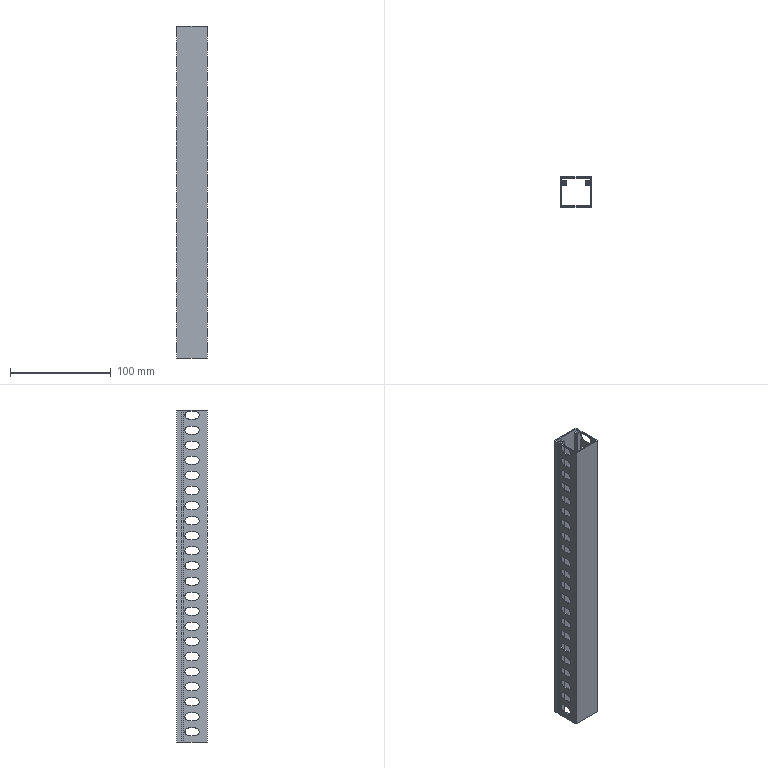Part | SolidWorks | features BaseBody 1 | 1 solid | 202 faces | box 30 x 30 x 330 mm | volume 40556 mm3 | plane 114 | cylinder 88 | commonest cylinder face diameters 8 x88